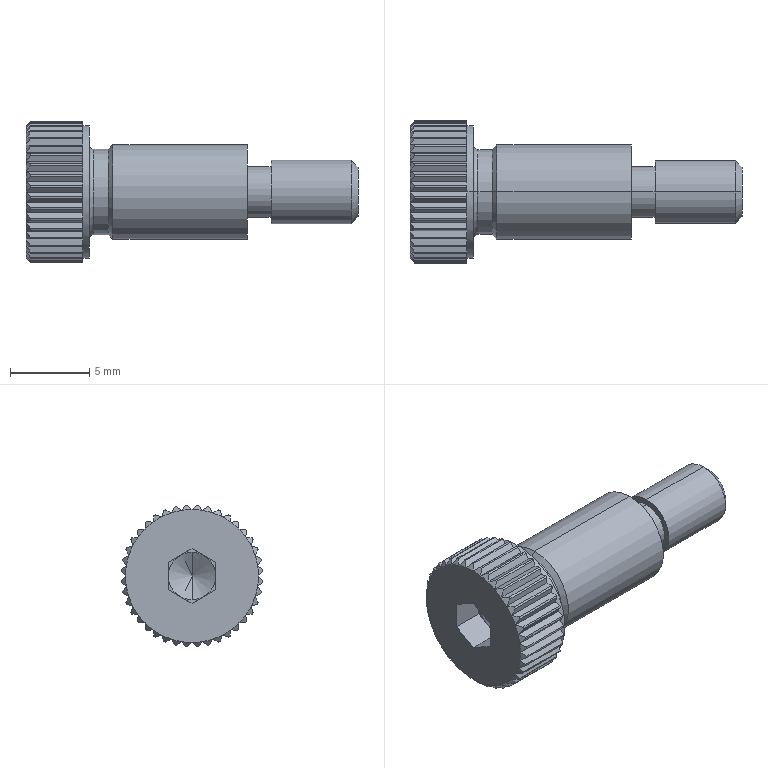Part | STEP file | 001-006-TBH02_d6_L10 | 1 solid | 235 faces | box 21 x 8.981 x 8.981 mm | volume 576.249 mm3 | plane 137 | cylinder 50 | cone 46 | torus 2 | commonest cylinder face diameters 9 x40 3.2 x2 4 x2 5.4 x2 6 x2 8.4 x2